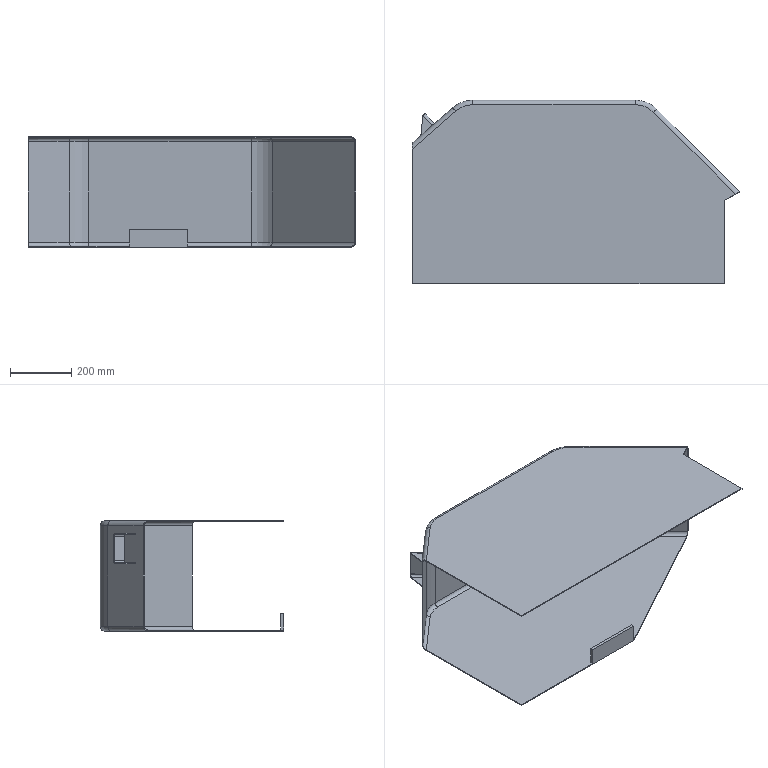Part | SolidWorks | 1 solid | 58 faces | box 1070 x 600 x 360 mm | volume 4618746 mm3 | plane 30 | cylinder 20 | torus 8 | commonest cylinder face diameters 24 x6 30 x6 14 x2 20 x2 194 x2 200 x2